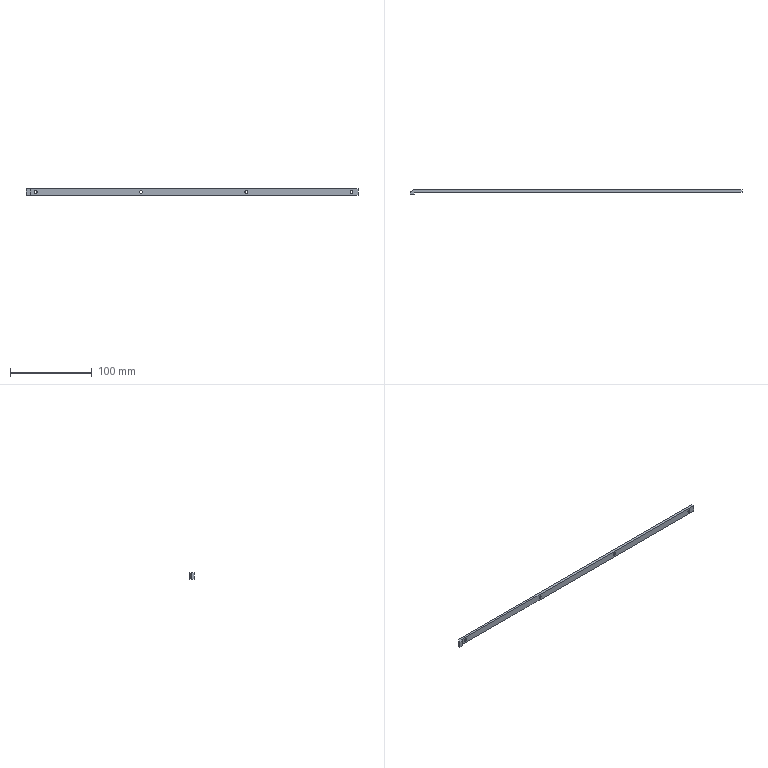Part | STEP file | CON-023 | 1 solid | 25 faces | box 405 x 5 x 8 mm | volume 9596 mm3 | plane 9 | cone 8 | cylinder 8 | commonest cylinder face diameters 3.4 x8